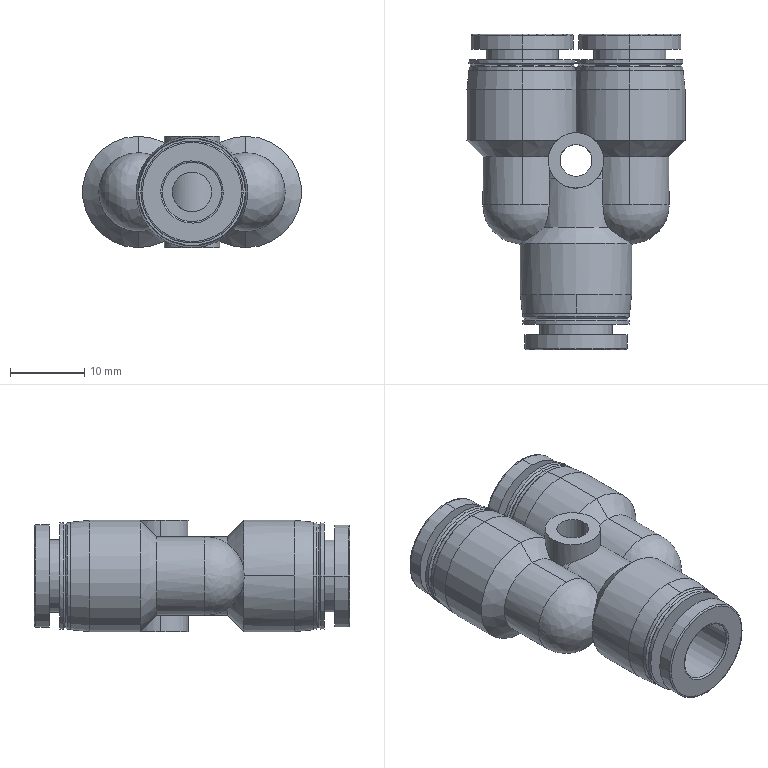Part | STEP file | 1 solid | 132 faces | box 29.502 x 42.5 x 15.002 mm | volume 6910 mm3 | cylinder 65 | cone 29 | spline 20 | plane 18 | commonest cylinder face diameters 14.4 x12 10.6 x11 7.478 x8 5.333 x6 8 x6 9.8 x6